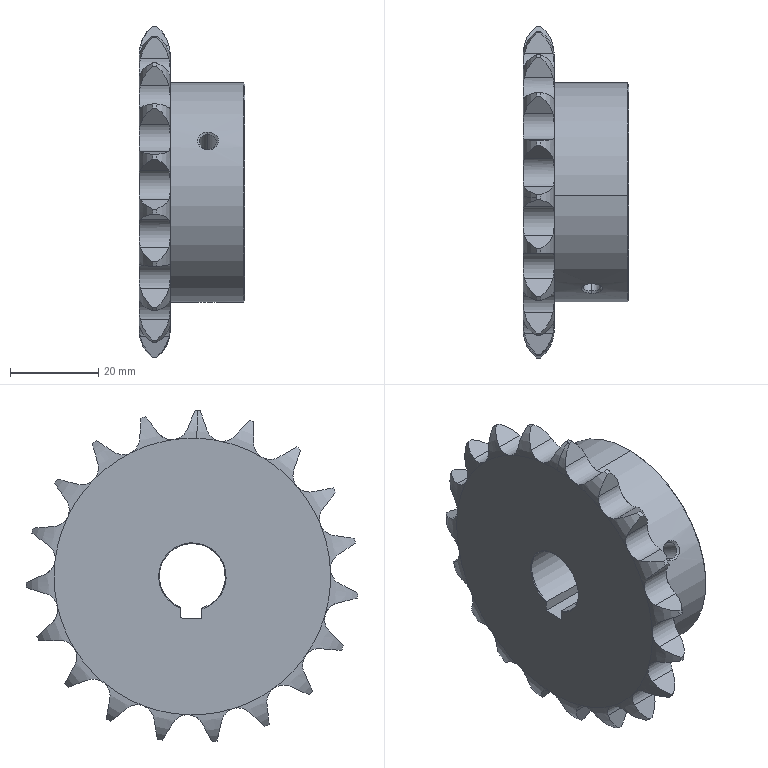Part | NX | 1 solid | 148 faces | box 24 x 75.39 x 75.33 mm | volume 52699 mm3 | cylinder 53 | plane 44 | torus 39 | cone 12 | commonest cylinder face diameters 7.62 x26 75.6 x19 3.84 x4 15 x2 49.8 x2